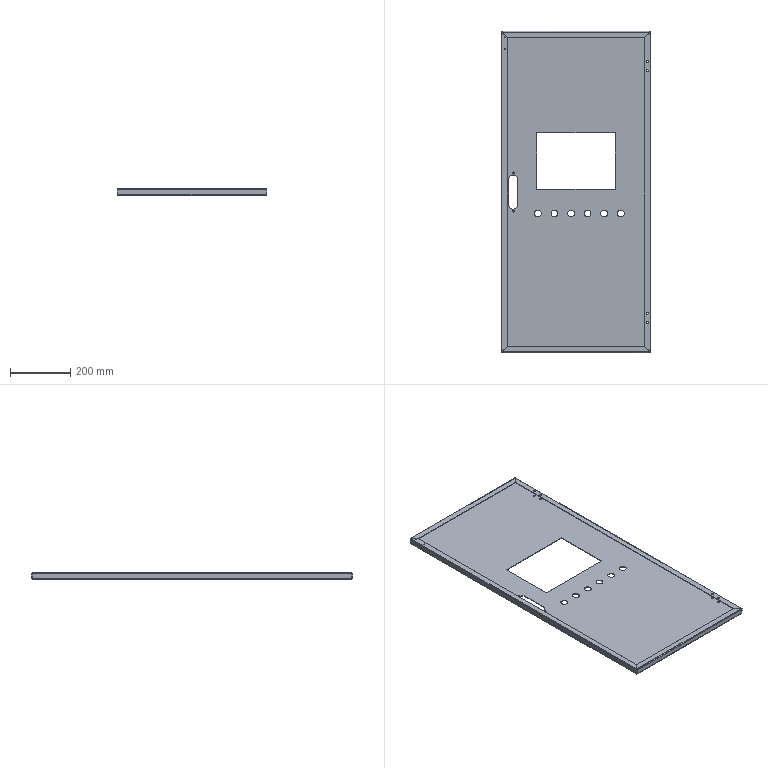Part | SolidWorks | features Cut 2, EdgeFlange 2, HoleWzd 2, ICE 2, LPattern 2, FlatPattern 1, SMBaseFlange 1, SheetMetal 1 | 1 solid | 114 faces | box 497 x 1066 x 20 mm | volume 1161554 mm3 | cylinder 54 | plane 44 | spline 16 | commonest cylinder face diameters 6.5 x16 22.5 x12 1.473 x8 5.473 x8 3.3 x4 7 x4